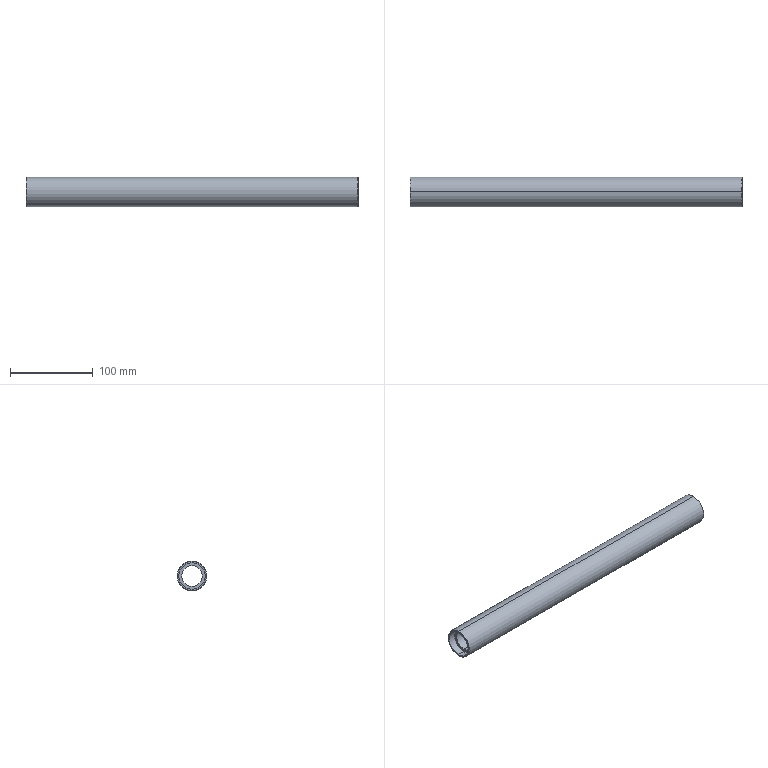Part | STEP file | PN_0018 | 1 solid | 16 faces | box 402 x 36 x 36 mm | volume 206186 mm3 | cylinder 8 | cone 4 | plane 4 | commonest cylinder face diameters 32 x4 25 x2 36 x2
STEP:
#1=CARTESIAN_POINT('',(0.,0.,0.));
#2=DIRECTION('',(0.,0.,1.));
#3=DIRECTION('',(1.,0.,0.));
#4=AXIS2_PLACEMENT_3D('',#1,#2,#3);
#5=CARTESIAN_POINT('',(-201.,0.,17.5));
#6=VERTEX_POINT('',#5);
#7=CARTESIAN_POINT('',(-201.,0.,-17.5));
#8=VERTEX_POINT('',#7);
#9=CARTESIAN_POINT('',(-201.,0.,0.));
#10=DIRECTION('',(-1.,0.,0.));
#11=DIRECTION('',(0.,0.,-1.));
#12=AXIS2_PLACEMENT_3D('',#9,#10,#11);
#13=CIRCLE('',#12,17.5);
#14=CARTESIAN_POINT('',(-201.,0.,0.));
#15=DIRECTION('',(1.,0.,0.));
#16=DIRECTION('',(0.,0.,-1.));
#17=AXIS2_PLACEMENT_3D('',#14,#15,#16);
#18=CONICAL_SURFACE('',#17,17.5,0.7854);
#19=CARTESIAN_POINT('',(6.283,0.));
#20=DIRECTION('',(-1.,0.));
#21=VECTOR('',#20,1.);
#22=LINE('',#19,#21);
#23=(GEOMETRIC_REPRESENTATION_CONTEXT(2)PARAMETRIC_REPRESENTATION_CONTEXT()REPRESENTATION_CONTEXT('',''));
#24=DEFINITIONAL_REPRESENTATION('',(#22),#23);
#25=PCURVE('',#18,#24);
#26=CARTESIAN_POINT('',(-201.,18.,0.));
#27=DIRECTION('',(1.,0.,0.));
#28=DIRECTION('',(0.,0.,-1.));
#29=AXIS2_PLACEMENT_3D('',#26,#27,#28);
#30=PLANE('',#29);
#31=CARTESIAN_POINT('',(17.5,-18.));
#32=CARTESIAN_POINT('',(17.5,-48.311));
#33=CARTESIAN_POINT('',(-8.75,-33.155));
#34=CARTESIAN_POINT('',(-35.,-18.));
#35=CARTESIAN_POINT('',(-8.75,-2.845));
#36=CARTESIAN_POINT('',(17.5,12.311));
#37=CARTESIAN_POINT('',(17.5,-18.));
#38=(BOUNDED_CURVE()B_SPLINE_CURVE(2,(#31,#32,#33,#34,#35,#36,#37),.UNSPECIFIED.,.T.,.F.)B_SPLINE_CURVE_WITH_KNOTS((1,2,2,2,2,1),(-2.094,0.,2.094,4.189,6.283,8.378),.UNSPECIFIED.)CURVE()GEOMETRIC_REPRESENTATION_ITEM()RATIONAL_B_SPLINE_CURVE((1.,0.5,1.,0.5,1.,0.5,1.))REPRESENTATION_ITEM(''));
#39=(GEOMETRIC_REPRESENTATION_CONTEXT(2)PARAMETRIC_REPRESENTATION_CONTEXT()REPRESENTATION_CONTEXT('',''));
#40=DEFINITIONAL_REPRESENTATION('',(#38),#39);
#41=PCURVE('',#30,#40);
#42=SURFACE_CURVE('',#13,(#25,#41),.PCURVE_S1.);
#43=EDGE_CURVE('',#6,#8,#42,.T.);
#44=ORIENTED_EDGE('',*,*,#43,.F.);
#45=CARTESIAN_POINT('',(-200.5,0.,18.));
#46=VERTEX_POINT('',#45);
#47=CARTESIAN_POINT('',(-201.,0.,17.5));
#48=DIRECTION('',(0.7071,0.,0.7071));
#49=VECTOR('',#48,1.);
#50=LINE('',#47,#49);
#51=CARTESIAN_POINT('',(3.142,0.));
#52=DIRECTION('',(0.,1.));
#53=VECTOR('',#52,1.);
#54=LINE('',#51,#53);
#55=(GEOMETRIC_REPRESENTATION_CONTEXT(2)PARAMETRIC_REPRESENTATION_CONTEXT()REPRESENTATION_CONTEXT('',''));
#56=DEFINITIONAL_REPRESENTATION('',(#54),#55);
#57=PCURVE('',#18,#56);
#58=CARTESIAN_POINT('',(-201.,0.,0.));
#59=DIRECTION('',(1.,0.,0.));
#60=DIRECTION('',(0.,0.,-1.));
#61=AXIS2_PLACEMENT_3D('',#58,#59,#60);
#62=CONICAL_SURFACE('',#61,17.5,0.7854);
#63=CARTESIAN_POINT('',(3.142,0.));
#64=DIRECTION('',(0.,1.));
#65=VECTOR('',#64,1.);
#66=LINE('',#63,#65);
#67=(GEOMETRIC_REPRESENTATION_CONTEXT(2)PARAMETRIC_REPRESENTATION_CONTEXT()REPRESENTATION_CONTEXT('',''));
#68=DEFINITIONAL_REPRESENTATION('',(#66),#67);
#69=PCURVE('',#62,#68);
#70=SURFACE_CURVE('',#50,(#57,#69),.PCURVE_S1.);
#71=EDGE_CURVE('',#6,#46,#70,.T.);
#72=ORIENTED_EDGE('',*,*,#71,.T.);
#73=CARTESIAN_POINT('',(-200.5,0.,-18.));
#74=VERTEX_POINT('',#73);
#75=CARTESIAN_POINT('',(-200.5,0.,0.));
#76=DIRECTION('',(1.,0.,0.));
#77=DIRECTION('',(0.,0.,-1.));
#78=AXIS2_PLACEMENT_3D('',#75,#76,#77);
#79=CIRCLE('',#78,18.);
#80=CARTESIAN_POINT('',(0.,0.5));
#81=DIRECTION('',(1.,0.));
#82=VECTOR('',#81,1.);
#83=LINE('',#80,#82);
#84=(GEOMETRIC_REPRESENTATION_CONTEXT(2)PARAMETRIC_REPRESENTATION_CONTEXT()REPRESENTATION_CONTEXT('',''));
#85=DEFINITIONAL_REPRESENTATION('',(#83),#84);
#86=PCURVE('',#18,#85);
#87=CARTESIAN_POINT('',(0.,0.,0.));
#88=DIRECTION('',(-1.,0.,0.));
#89=DIRECTION('',(0.,0.,1.));
#90=AXIS2_PLACEMENT_3D('',#87,#88,#89);
#91=CYLINDRICAL_SURFACE('',#90,18.);
#92=CARTESIAN_POINT('',(3.142,200.5));
#93=DIRECTION('',(-1.,0.));
#94=VECTOR('',#93,1.);
#95=LINE('',#92,#94);
#96=(GEOMETRIC_REPRESENTATION_CONTEXT(2)PARAMETRIC_REPRESENTATION_CONTEXT()REPRESENTATION_CONTEXT('',''));
#97=DEFINITIONAL_REPRESENTATION('',(#95),#96);
#98=PCURVE('',#91,#97);
#99=SURFACE_CURVE('',#79,(#86,#98),.PCURVE_S1.);
#100=EDGE_CURVE('',#74,#46,#99,.T.);
#101=ORIENTED_EDGE('',*,*,#100,.F.);
#102=CARTESIAN_POINT('',(-201.,0.,-17.5));
#103=DIRECTION('',(0.7071,0.,-0.7071));
#104=VECTOR('',#103,1.);
#105=LINE('',#102,#104);
#106=CARTESIAN_POINT('',(0.,0.));
#107=DIRECTION('',(0.,1.));
#108=VECTOR('',#107,1.);
#109=LINE('',#106,#108);
#110=(GEOMETRIC_REPRESENTATION_CONTEXT(2)PARAMETRIC_REPRESENTATION_CONTEXT()REPRESENTATION_CONTEXT('',''));
#111=DEFINITIONAL_REPRESENTATION('',(#109),#110);
#112=PCURVE('',#18,#111);
#113=CARTESIAN_POINT('',(6.283,0.));
#114=DIRECTION('',(0.,1.));
#115=VECTOR('',#114,1.);
#116=LINE('',#113,#115);
#117=(GEOMETRIC_REPRESENTATION_CONTEXT(2)PARAMETRIC_REPRESENTATION_CONTEXT()REPRESENTATION_CONTEXT('',''));
#118=DEFINITIONAL_REPRESENTATION('',(#116),#117);
#119=PCURVE('',#62,#118);
#120=SURFACE_CURVE('',#105,(#112,#119),.PCURVE_S1.);
#121=EDGE_CURVE('',#8,#74,#120,.T.);
#122=ORIENTED_EDGE('',*,*,#121,.F.);
#123=EDGE_LOOP('',(#44,#72,#101,#122));
#124=FACE_BOUND('',#123,.T.);
#125=ADVANCED_FACE('',(#124),#18,.T.);
#126=CARTESIAN_POINT('',(201.,0.,-17.5));
#127=VERTEX_POINT('',#126);
#128=CARTESIAN_POINT('',(201.,0.,17.5));
#129=VERTEX_POINT('',#128);
#130=CARTESIAN_POINT('',(201.,0.,0.));
#131=DIRECTION('',(1.,0.,0.));
#132=DIRECTION('',(0.,0.,1.));
#133=AXIS2_PLACEMENT_3D('',#130,#131,#132);
#134=CIRCLE('',#133,17.5);
#135=CARTESIAN_POINT('',(200.5,0.,0.));
#136=DIRECTION('',(-1.,0.,0.));
#137=DIRECTION('',(0.,0.,1.));
#138=AXIS2_PLACEMENT_3D('',#135,#136,#137);
#139=CONICAL_SURFACE('',#138,18.,0.7854);
#140=CARTESIAN_POINT('',(6.283,-0.5));
#141=DIRECTION('',(-1.,0.));
#142=VECTOR('',#141,1.);
#143=LINE('',#140,#142);
#144=(GEOMETRIC_REPRESENTATION_CONTEXT(2)PARAMETRIC_REPRESENTATION_CONTEXT()REPRESENTATION_CONTEXT('',''));
#145=DEFINITIONAL_REPRESENTATION('',(#143),#144);
#146=PCURVE('',#139,#145);
#147=CARTESIAN_POINT('',(201.,18.,0.));
#148=DIRECTION('',(-1.,0.,0.));
#149=DIRECTION('',(0.,0.,1.));
#150=AXIS2_PLACEMENT_3D('',#147,#148,#149);
#151=PLANE('',#150);
#152=CARTESIAN_POINT('',(17.5,-18.));
#153=CARTESIAN_POINT('',(17.5,-48.311));
#154=CARTESIAN_POINT('',(-8.75,-33.155));
#155=CARTESIAN_POINT('',(-35.,-18.));
#156=CARTESIAN_POINT('',(-8.75,-2.845));
#157=CARTESIAN_POINT('',(17.5,12.311));
#158=CARTESIAN_POINT('',(17.5,-18.));
#159=(BOUNDED_CURVE()B_SPLINE_CURVE(2,(#152,#153,#154,#155,#156,#157,#158),.UNSPECIFIED.,.T.,.F.)B_SPLINE_CURVE_WITH_KNOTS((1,2,2,2,2,1),(-2.094,0.,2.094,4.189,6.283,8.378),.UNSPECIFIED.)CURVE()GEOMETRIC_REPRESENTATION_ITEM()RATIONAL_B_SPLINE_CURVE((1.,0.5,1.,0.5,1.,0.5,1.))REPRESENTATION_ITEM(''));
#160=(GEOMETRIC_REPRESENTATION_CONTEXT(2)PARAMETRIC_REPRESENTATION_CONTEXT()REPRESENTATION_CONTEXT('',''));
#161=DEFINITIONAL_REPRESENTATION('',(#159),#160);
#162=PCURVE('',#151,#161);
#163=SURFACE_CURVE('',#134,(#146,#162),.PCURVE_S1.);
#164=EDGE_CURVE('',#127,#129,#163,.T.);
#165=ORIENTED_EDGE('',*,*,#164,.F.);
#166=CARTESIAN_POINT('',(200.5,0.,-18.));
#167=VERTEX_POINT('',#166);
#168=CARTESIAN_POINT('',(200.5,0.,-18.));
#169=DIRECTION('',(-0.7071,0.,-0.7071));
#170=VECTOR('',#169,1.);
#171=LINE('',#168,#170);
#172=CARTESIAN_POINT('',(3.142,0.));
#173=DIRECTION('',(0.,1.));
#174=VECTOR('',#173,1.);
#175=LINE('',#172,#174);
#176=(GEOMETRIC_REPRESENTATION_CONTEXT(2)PARAMETRIC_REPRESENTATION_CONTEXT()REPRESENTATION_CONTEXT('',''));
#177=DEFINITIONAL_REPRESENTATION('',(#175),#176);
#178=PCURVE('',#139,#177);
#179=CARTESIAN_POINT('',(200.5,0.,0.));
#180=DIRECTION('',(-1.,0.,0.));
#181=DIRECTION('',(0.,0.,1.));
#182=AXIS2_PLACEMENT_3D('',#179,#180,#181);
#183=CONICAL_SURFACE('',#182,18.,0.7854);
#184=CARTESIAN_POINT('',(3.142,0.));
#185=DIRECTION('',(0.,1.));
#186=VECTOR('',#185,1.);
#187=LINE('',#184,#186);
#188=(GEOMETRIC_REPRESENTATION_CONTEXT(2)PARAMETRIC_REPRESENTATION_CONTEXT()REPRESENTATION_CONTEXT('',''));
#189=DEFINITIONAL_REPRESENTATION('',(#187),#188);
#190=PCURVE('',#183,#189);
#191=SURFACE_CURVE('',#171,(#178,#190),.PCURVE_S1.);
#192=EDGE_CURVE('',#127,#167,#191,.T.);
#193=ORIENTED_EDGE('',*,*,#192,.T.);
#194=CARTESIAN_POINT('',(200.5,0.,18.));
#195=VERTEX_POINT('',#194);
#196=CARTESIAN_POINT('',(200.5,0.,0.));
#197=DIRECTION('',(-1.,0.,0.));
#198=DIRECTION('',(0.,0.,1.));
#199=AXIS2_PLACEMENT_3D('',#196,#197,#198);
#200=CIRCLE('',#199,18.);
#201=CARTESIAN_POINT('',(0.,0.));
#202=DIRECTION('',(1.,0.));
#203=VECTOR('',#202,1.);
#204=LINE('',#201,#203);
#205=(GEOMETRIC_REPRESENTATION_CONTEXT(2)PARAMETRIC_REPRESENTATION_CONTEXT()REPRESENTATION_CONTEXT('',''));
#206=DEFINITIONAL_REPRESENTATION('',(#204),#205);
#207=PCURVE('',#139,#206);
#208=CARTESIAN_POINT('',(0.,-200.5));
#209=DIRECTION('',(1.,0.));
#210=VECTOR('',#209,1.);
#211=LINE('',#208,#210);
#212=(GEOMETRIC_REPRESENTATION_CONTEXT(2)PARAMETRIC_REPRESENTATION_CONTEXT()REPRESENTATION_CONTEXT('',''));
#213=DEFINITIONAL_REPRESENTATION('',(#211),#212);
#214=PCURVE('',#91,#213);
#215=SURFACE_CURVE('',#200,(#207,#214),.PCURVE_S1.);
#216=EDGE_CURVE('',#195,#167,#215,.T.);
#217=ORIENTED_EDGE('',*,*,#216,.F.);
#218=CARTESIAN_POINT('',(200.5,0.,18.));
#219=DIRECTION('',(-0.7071,0.,0.7071));
#220=VECTOR('',#219,1.);
#221=LINE('',#218,#220);
#222=CARTESIAN_POINT('',(0.,0.));
#223=DIRECTION('',(0.,1.));
#224=VECTOR('',#223,1.);
#225=LINE('',#222,#224);
#226=(GEOMETRIC_REPRESENTATION_CONTEXT(2)PARAMETRIC_REPRESENTATION_CONTEXT()REPRESENTATION_CONTEXT('',''));
#227=DEFINITIONAL_REPRESENTATION('',(#225),#226);
#228=PCURVE('',#139,#227);
#229=CARTESIAN_POINT('',(6.283,0.));
#230=DIRECTION('',(0.,1.));
#231=VECTOR('',#230,1.);
#232=LINE('',#229,#231);
#233=(GEOMETRIC_REPRESENTATION_CONTEXT(2)PARAMETRIC_REPRESENTATION_CONTEXT()REPRESENTATION_CONTEXT('',''));
#234=DEFINITIONAL_REPRESENTATION('',(#232),#233);
#235=PCURVE('',#183,#234);
#236=SURFACE_CURVE('',#221,(#228,#235),.PCURVE_S1.);
#237=EDGE_CURVE('',#129,#195,#236,.T.);
#238=ORIENTED_EDGE('',*,*,#237,.F.);
#239=EDGE_LOOP('',(#165,#193,#217,#238));
#240=FACE_BOUND('',#239,.T.);
#241=ADVANCED_FACE('',(#240),#139,.T.);
#242=CARTESIAN_POINT('',(192.,0.,12.5));
#243=VERTEX_POINT('',#242);
#244=CARTESIAN_POINT('',(-192.,0.,12.5));
#245=VERTEX_POINT('',#244);
#246=CARTESIAN_POINT('',(0.,0.,12.5));
#247=DIRECTION('',(-1.,0.,0.));
#248=VECTOR('',#247,1.);
#249=LINE('',#246,#248);
#250=CARTESIAN_POINT('',(0.,0.,0.));
#251=DIRECTION('',(-1.,0.,0.));
#252=DIRECTION('',(0.,0.,1.));
#253=AXIS2_PLACEMENT_3D('',#250,#251,#252);
#254=CYLINDRICAL_SURFACE('',#253,12.5);
#255=CARTESIAN_POINT('',(6.283,0.));
#256=DIRECTION('',(0.,1.));
#257=VECTOR('',#256,1.);
#258=LINE('',#255,#257);
#259=(GEOMETRIC_REPRESENTATION_CONTEXT(2)PARAMETRIC_REPRESENTATION_CONTEXT()REPRESENTATION_CONTEXT('',''));
#260=DEFINITIONAL_REPRESENTATION('',(#258),#259);
#261=PCURVE('',#254,#260);
#262=CARTESIAN_POINT('',(0.,0.,0.));
#263=DIRECTION('',(-1.,0.,0.));
#264=DIRECTION('',(0.,0.,1.));
#265=AXIS2_PLACEMENT_3D('',#262,#263,#264);
#266=CYLINDRICAL_SURFACE('',#265,12.5);
#267=CARTESIAN_POINT('',(0.,0.));
#268=DIRECTION('',(0.,1.));
#269=VECTOR('',#268,1.);
#270=LINE('',#267,#269);
#271=(GEOMETRIC_REPRESENTATION_CONTEXT(2)PARAMETRIC_REPRESENTATION_CONTEXT()REPRESENTATION_CONTEXT('',''));
#272=DEFINITIONAL_REPRESENTATION('',(#270),#271);
#273=PCURVE('',#266,#272);
#274=SURFACE_CURVE('',#249,(#261,#273),.PCURVE_S1.);
#275=EDGE_CURVE('',#243,#245,#274,.T.);
#276=ORIENTED_EDGE('',*,*,#275,.T.);
#277=CARTESIAN_POINT('',(-192.,0.,-12.5));
#278=VERTEX_POINT('',#277);
#279=CARTESIAN_POINT('',(-192.,0.,0.));
#280=DIRECTION('',(-1.,0.,0.));
#281=DIRECTION('',(0.,0.,1.));
#282=AXIS2_PLACEMENT_3D('',#279,#280,#281);
#283=CIRCLE('',#282,12.5);
#284=CARTESIAN_POINT('',(0.,192.));
#285=DIRECTION('',(1.,0.));
#286=VECTOR('',#285,1.);
#287=LINE('',#284,#286);
#288=(GEOMETRIC_REPRESENTATION_CONTEXT(2)PARAMETRIC_REPRESENTATION_CONTEXT()REPRESENTATION_CONTEXT('',''));
#289=DEFINITIONAL_REPRESENTATION('',(#287),#288);
#290=PCURVE('',#254,#289);
#291=CARTESIAN_POINT('',(-192.,16.,0.));
#292=DIRECTION('',(1.,0.,0.));
#293=DIRECTION('',(0.,0.,-1.));
#294=AXIS2_PLACEMENT_3D('',#291,#292,#293);
#295=PLANE('',#294);
#296=CARTESIAN_POINT('',(-12.5,-16.));
#297=CARTESIAN_POINT('',(-12.5,5.651));
#298=CARTESIAN_POINT('',(6.25,-5.175));
#299=CARTESIAN_POINT('',(25.,-16.));
#300=CARTESIAN_POINT('',(6.25,-26.825));
#301=CARTESIAN_POINT('',(-12.5,-37.651));
#302=CARTESIAN_POINT('',(-12.5,-16.));
#303=(BOUNDED_CURVE()B_SPLINE_CURVE(2,(#296,#297,#298,#299,#300,#301,#302),.UNSPECIFIED.,.T.,.F.)B_SPLINE_CURVE_WITH_KNOTS((1,2,2,2,2,1),(-2.094,0.,2.094,4.189,6.283,8.378),.UNSPECIFIED.)CURVE()GEOMETRIC_REPRESENTATION_ITEM()RATIONAL_B_SPLINE_CURVE((1.,0.5,1.,0.5,1.,0.5,1.))REPRESENTATION_ITEM(''));
#304=(GEOMETRIC_REPRESENTATION_CONTEXT(2)PARAMETRIC_REPRESENTATION_CONTEXT()REPRESENTATION_CONTEXT('',''));
#305=DEFINITIONAL_REPRESENTATION('',(#303),#304);
#306=PCURVE('',#295,#305);
#307=SURFACE_CURVE('',#283,(#290,#306),.PCURVE_S1.);
#308=EDGE_CURVE('',#278,#245,#307,.T.);
#309=ORIENTED_EDGE('',*,*,#308,.F.);
#310=CARTESIAN_POINT('',(192.,0.,-12.5));
#311=VERTEX_POINT('',#310);
#312=CARTESIAN_POINT('',(0.,0.,-12.5));
#313=DIRECTION('',(-1.,0.,0.));
#314=VECTOR('',#313,1.);
#315=LINE('',#312,#314);
#316=CARTESIAN_POINT('',(3.142,0.));
#317=DIRECTION('',(0.,1.));
#318=VECTOR('',#317,1.);
#319=LINE('',#316,#318);
#320=(GEOMETRIC_REPRESENTATION_CONTEXT(2)PARAMETRIC_REPRESENTATION_CONTEXT()REPRESENTATION_CONTEXT('',''));
#321=DEFINITIONAL_REPRESENTATION('',(#319),#320);
#322=PCURVE('',#254,#321);
#323=CARTESIAN_POINT('',(3.142,0.));
#324=DIRECTION('',(0.,1.));
#325=VECTOR('',#324,1.);
#326=LINE('',#323,#325);
#327=(GEOMETRIC_REPRESENTATION_CONTEXT(2)PARAMETRIC_REPRESENTATION_CONTEXT()REPRESENTATION_CONTEXT('',''));
#328=DEFINITIONAL_REPRESENTATION('',(#326),#327);
#329=PCURVE('',#266,#328);
#330=SURFACE_CURVE('',#315,(#322,#329),.PCURVE_S1.);
#331=EDGE_CURVE('',#311,#278,#330,.T.);
#332=ORIENTED_EDGE('',*,*,#331,.F.);
#333=CARTESIAN_POINT('',(192.,0.,0.));
#334=DIRECTION('',(-1.,0.,0.));
#335=DIRECTION('',(0.,0.,1.));
#336=AXIS2_PLACEMENT_3D('',#333,#334,#335);
#337=CIRCLE('',#336,12.5);
#338=CARTESIAN_POINT('',(0.,-192.));
#339=DIRECTION('',(1.,0.));
#340=VECTOR('',#339,1.);
#341=LINE('',#338,#340);
#342=(GEOMETRIC_REPRESENTATION_CONTEXT(2)PARAMETRIC_REPRESENTATION_CONTEXT()REPRESENTATION_CONTEXT('',''));
#343=DEFINITIONAL_REPRESENTATION('',(#341),#342);
#344=PCURVE('',#254,#343);
#345=CARTESIAN_POINT('',(192.,16.,0.));
#346=DIRECTION('',(-1.,0.,0.));
#347=DIRECTION('',(0.,0.,1.));
#348=AXIS2_PLACEMENT_3D('',#345,#346,#347);
#349=PLANE('',#348);
#350=CARTESIAN_POINT('',(0.,-16.));
#351=DIRECTION('',(1.,0.));
#352=AXIS2_PLACEMENT_2D('',#350,#351);
#353=CIRCLE('',#352,12.5);
#354=(GEOMETRIC_REPRESENTATION_CONTEXT(2)PARAMETRIC_REPRESENTATION_CONTEXT()REPRESENTATION_CONTEXT('',''));
#355=DEFINITIONAL_REPRESENTATION('',(#353),#354);
#356=PCURVE('',#349,#355);
#357=SURFACE_CURVE('',#337,(#344,#356),.PCURVE_S1.);
#358=EDGE_CURVE('',#311,#243,#357,.T.);
#359=ORIENTED_EDGE('',*,*,#358,.T.);
#360=EDGE_LOOP('',(#276,#309,#332,#359));
#361=FACE_BOUND('',#360,.F.);
#362=ADVANCED_FACE('',(#361),#254,.F.);
#363=CARTESIAN_POINT('',(201.,0.,16.));
#364=VERTEX_POINT('',#363);
#365=CARTESIAN_POINT('',(192.,0.,16.));
#366=VERTEX_POINT('',#365);
#367=CARTESIAN_POINT('',(0.,0.,16.));
#368=DIRECTION('',(-1.,0.,0.));
#369=VECTOR('',#368,1.);
#370=LINE('',#367,#369);
#371=CARTESIAN_POINT('',(0.,0.,0.));
#372=DIRECTION('',(-1.,0.,0.));
#373=DIRECTION('',(0.,0.,1.));
#374=AXIS2_PLACEMENT_3D('',#371,#372,#373);
#375=CYLINDRICAL_SURFACE('',#374,16.);
#376=CARTESIAN_POINT('',(6.283,0.));
#377=DIRECTION('',(0.,1.));
#378=VECTOR('',#377,1.);
#379=LINE('',#376,#378);
#380=(GEOMETRIC_REPRESENTATION_CONTEXT(2)PARAMETRIC_REPRESENTATION_CONTEXT()REPRESENTATION_CONTEXT('',''));
#381=DEFINITIONAL_REPRESENTATION('',(#379),#380);
#382=PCURVE('',#375,#381);
#383=CARTESIAN_POINT('',(0.,0.,0.));
#384=DIRECTION('',(-1.,0.,0.));
#385=DIRECTION('',(0.,0.,1.));
#386=AXIS2_PLACEMENT_3D('',#383,#384,#385);
#387=CYLINDRICAL_SURFACE('',#386,16.);
#388=CARTESIAN_POINT('',(0.,0.));
#389=DIRECTION('',(0.,1.));
#390=VECTOR('',#389,1.);
#391=LINE('',#388,#390);
#392=(GEOMETRIC_REPRESENTATION_CONTEXT(2)PARAMETRIC_REPRESENTATION_CONTEXT()REPRESENTATION_CONTEXT('',''));
#393=DEFINITIONAL_REPRESENTATION('',(#391),#392);
#394=PCURVE('',#387,#393);
#395=SURFACE_CURVE('',#370,(#382,#394),.PCURVE_S1.);
#396=EDGE_CURVE('',#364,#366,#395,.T.);
#397=ORIENTED_EDGE('',*,*,#396,.T.);
#398=CARTESIAN_POINT('',(192.,0.,-16.));
#399=VERTEX_POINT('',#398);
#400=CARTESIAN_POINT('',(192.,0.,0.));
#401=DIRECTION('',(-1.,0.,0.));
#402=DIRECTION('',(0.,0.,1.));
#403=AXIS2_PLACEMENT_3D('',#400,#401,#402);
#404=CIRCLE('',#403,16.);
#405=CARTESIAN_POINT('',(0.,-192.));
#406=DIRECTION('',(1.,0.));
#407=VECTOR('',#406,1.);
#408=LINE('',#405,#407);
#409=(GEOMETRIC_REPRESENTATION_CONTEXT(2)PARAMETRIC_REPRESENTATION_CONTEXT()REPRESENTATION_CONTEXT('',''));
#410=DEFINITIONAL_REPRESENTATION('',(#408),#409);
#411=PCURVE('',#375,#410);
#412=CARTESIAN_POINT('',(0.,-16.));
#413=DIRECTION('',(1.,0.));
#414=AXIS2_PLACEMENT_2D('',#412,#413);
#415=CIRCLE('',#414,16.);
#416=(GEOMETRIC_REPRESENTATION_CONTEXT(2)PARAMETRIC_REPRESENTATION_CONTEXT()REPRESENTATION_CONTEXT('',''));
#417=DEFINITIONAL_REPRESENTATION('',(#415),#416);
#418=PCURVE('',#349,#417);
#419=SURFACE_CURVE('',#404,(#411,#418),.PCURVE_S1.);
#420=EDGE_CURVE('',#399,#366,#419,.T.);
#421=ORIENTED_EDGE('',*,*,#420,.F.);
#422=CARTESIAN_POINT('',(201.,0.,-16.));
#423=VERTEX_POINT('',#422);
#424=CARTESIAN_POINT('',(0.,0.,-16.));
#425=DIRECTION('',(-1.,0.,0.));
#426=VECTOR('',#425,1.);
#427=LINE('',#424,#426);
#428=CARTESIAN_POINT('',(3.142,0.));
#429=DIRECTION('',(0.,1.));
#430=VECTOR('',#429,1.);
#431=LINE('',#428,#430);
#432=(GEOMETRIC_REPRESENTATION_CONTEXT(2)PARAMETRIC_REPRESENTATION_CONTEXT()REPRESENTATION_CONTEXT('',''));
#433=DEFINITIONAL_REPRESENTATION('',(#431),#432);
#434=PCURVE('',#375,#433);
#435=CARTESIAN_POINT('',(3.142,0.));
#436=DIRECTION('',(0.,1.));
#437=VECTOR('',#436,1.);
#438=LINE('',#435,#437);
#439=(GEOMETRIC_REPRESENTATION_CONTEXT(2)PARAMETRIC_REPRESENTATION_CONTEXT()REPRESENTATION_CONTEXT('',''));
#440=DEFINITIONAL_REPRESENTATION('',(#438),#439);
#441=PCURVE('',#387,#440);
#442=SURFACE_CURVE('',#427,(#434,#441),.PCURVE_S1.);
#443=EDGE_CURVE('',#423,#399,#442,.T.);
#444=ORIENTED_EDGE('',*,*,#443,.F.);
#445=CARTESIAN_POINT('',(201.,0.,0.));
#446=DIRECTION('',(-1.,0.,0.));
#447=DIRECTION('',(0.,0.,1.));
#448=AXIS2_PLACEMENT_3D('',#445,#446,#447);
#449=CIRCLE('',#448,16.);
#450=CARTESIAN_POINT('',(0.,-201.));
#451=DIRECTION('',(1.,0.));
#452=VECTOR('',#451,1.);
#453=LINE('',#450,#452);
#454=(GEOMETRIC_REPRESENTATION_CONTEXT(2)PARAMETRIC_REPRESENTATION_CONTEXT()REPRESENTATION_CONTEXT('',''));
#455=DEFINITIONAL_REPRESENTATION('',(#453),#454);
#456=PCURVE('',#375,#455);
#457=CARTESIAN_POINT('',(0.,-18.));
#458=DIRECTION('',(1.,0.));
#459=AXIS2_PLACEMENT_2D('',#457,#458);
#460=CIRCLE('',#459,16.);
#461=(GEOMETRIC_REPRESENTATION_CONTEXT(2)PARAMETRIC_REPRESENTATION_CONTEXT()REPRESENTATION_CONTEXT('',''));
#462=DEFINITIONAL_REPRESENTATION('',(#460),#461);
#463=PCURVE('',#151,#462);
#464=SURFACE_CURVE('',#449,(#456,#463),.PCURVE_S1.);
#465=EDGE_CURVE('',#423,#364,#464,.T.);
#466=ORIENTED_EDGE('',*,*,#465,.T.);
#467=EDGE_LOOP('',(#397,#421,#444,#466));
#468=FACE_BOUND('',#467,.F.);
#469=ADVANCED_FACE('',(#468),#375,.F.);
#470=ORIENTED_EDGE('',*,*,#216,.T.);
#471=CARTESIAN_POINT('',(0.,0.,-18.));
#472=DIRECTION('',(-1.,0.,0.));
#473=VECTOR('',#472,1.);
#474=LINE('',#471,#473);
#475=CARTESIAN_POINT('',(3.142,0.));
#476=DIRECTION('',(0.,1.));
#477=VECTOR('',#476,1.);
#478=LINE('',#475,#477);
#479=(GEOMETRIC_REPRESENTATION_CONTEXT(2)PARAMETRIC_REPRESENTATION_CONTEXT()REPRESENTATION_CONTEXT('',''));
#480=DEFINITIONAL_REPRESENTATION('',(#478),#479);
#481=PCURVE('',#91,#480);
#482=CARTESIAN_POINT('',(0.,0.,0.));
#483=DIRECTION('',(-1.,0.,0.));
#484=DIRECTION('',(0.,0.,1.));
#485=AXIS2_PLACEMENT_3D('',#482,#483,#484);
#486=CYLINDRICAL_SURFACE('',#485,18.);
#487=CARTESIAN_POINT('',(3.142,0.));
#488=DIRECTION('',(0.,1.));
#489=VECTOR('',#488,1.);
#490=LINE('',#487,#489);
#491=(GEOMETRIC_REPRESENTATION_CONTEXT(2)PARAMETRIC_REPRESENTATION_CONTEXT()REPRESENTATION_CONTEXT('',''));
#492=DEFINITIONAL_REPRESENTATION('',(#490),#491);
#493=PCURVE('',#486,#492);
#494=SURFACE_CURVE('',#474,(#481,#493),.PCURVE_S1.);
#495=EDGE_CURVE('',#167,#74,#494,.T.);
#496=ORIENTED_EDGE('',*,*,#495,.T.);
#497=ORIENTED_EDGE('',*,*,#100,.T.);
#498=CARTESIAN_POINT('',(0.,0.,18.));
#499=DIRECTION('',(-1.,0.,0.));
#500=VECTOR('',#499,1.);
#501=LINE('',#498,#500);
#502=CARTESIAN_POINT('',(0.,0.));
#503=DIRECTION('',(0.,1.));
#504=VECTOR('',#503,1.);
#505=LINE('',#502,#504);
#506=(GEOMETRIC_REPRESENTATION_CONTEXT(2)PARAMETRIC_REPRESENTATION_CONTEXT()REPRESENTATION_CONTEXT('',''));
#507=DEFINITIONAL_REPRESENTATION('',(#505),#506);
#508=PCURVE('',#91,#507);
#509=CARTESIAN_POINT('',(6.283,0.));
#510=DIRECTION('',(0.,1.));
#511=VECTOR('',#510,1.);
#512=LINE('',#509,#511);
#513=(GEOMETRIC_REPRESENTATION_CONTEXT(2)PARAMETRIC_REPRESENTATION_CONTEXT()REPRESENTATION_CONTEXT('',''));
#514=DEFINITIONAL_REPRESENTATION('',(#512),#513);
#515=PCURVE('',#486,#514);
#516=SURFACE_CURVE('',#501,(#508,#515),.PCURVE_S1.);
#517=EDGE_CURVE('',#195,#46,#516,.T.);
#518=ORIENTED_EDGE('',*,*,#517,.F.);
#519=EDGE_LOOP('',(#470,#496,#497,#518));
#520=FACE_BOUND('',#519,.T.);
#521=ADVANCED_FACE('',(#520),#91,.T.);
#522=CARTESIAN_POINT('',(-192.,0.,16.));
#523=VERTEX_POINT('',#522);
#524=CARTESIAN_POINT('',(-201.,0.,16.));
#525=VERTEX_POINT('',#524);
#526=CARTESIAN_POINT('',(0.,0.,16.));
#527=DIRECTION('',(-1.,0.,0.));
#528=VECTOR('',#527,1.);
#529=LINE('',#526,#528);
#530=CARTESIAN_POINT('',(0.,0.,0.));
#531=DIRECTION('',(-1.,0.,0.));
#532=DIRECTION('',(0.,0.,1.));
#533=AXIS2_PLACEMENT_3D('',#530,#531,#532);
#534=CYLINDRICAL_SURFACE('',#533,16.);
#535=CARTESIAN_POINT('',(6.283,0.));
#536=DIRECTION('',(0.,1.));
#537=VECTOR('',#536,1.);
#538=LINE('',#535,#537);
#539=(GEOMETRIC_REPRESENTATION_CONTEXT(2)PARAMETRIC_REPRESENTATION_CONTEXT()REPRESENTATION_CONTEXT('',''));
#540=DEFINITIONAL_REPRESENTATION('',(#538),#539);
#541=PCURVE('',#534,#540);
#542=CARTESIAN_POINT('',(0.,0.,0.));
#543=DIRECTION('',(-1.,0.,0.));
#544=DIRECTION('',(0.,0.,1.));
#545=AXIS2_PLACEMENT_3D('',#542,#543,#544);
#546=CYLINDRICAL_SURFACE('',#545,16.);
#547=CARTESIAN_POINT('',(0.,0.));
#548=DIRECTION('',(0.,1.));
#549=VECTOR('',#548,1.);
#550=LINE('',#547,#549);
#551=(GEOMETRIC_REPRESENTATION_CONTEXT(2)PARAMETRIC_REPRESENTATION_CONTEXT()REPRESENTATION_CONTEXT('',''));
#552=DEFINITIONAL_REPRESENTATION('',(#550),#551);
#553=PCURVE('',#546,#552);
#554=SURFACE_CURVE('',#529,(#541,#553),.PCURVE_S1.);
#555=EDGE_CURVE('',#523,#525,#554,.T.);
#556=ORIENTED_EDGE('',*,*,#555,.T.);
#557=CARTESIAN_POINT('',(-201.,0.,-16.));
#558=VERTEX_POINT('',#557);
#559=CARTESIAN_POINT('',(-201.,0.,0.));
#560=DIRECTION('',(-1.,0.,0.));
#561=DIRECTION('',(0.,0.,1.));
#562=AXIS2_PLACEMENT_3D('',#559,#560,#561);
#563=CIRCLE('',#562,16.);
#564=CARTESIAN_POINT('',(0.,201.));
#565=DIRECTION('',(1.,0.));
#566=VECTOR('',#565,1.);
#567=LINE('',#564,#566);
#568=(GEOMETRIC_REPRESENTATION_CONTEXT(2)PARAMETRIC_REPRESENTATION_CONTEXT()REPRESENTATION_CONTEXT('',''));
#569=DEFINITIONAL_REPRESENTATION('',(#567),#568);
#570=PCURVE('',#534,#569);
#571=CARTESIAN_POINT('',(-16.,-18.));
#572=CARTESIAN_POINT('',(-16.,9.713));
#573=CARTESIAN_POINT('',(8.,-4.144));
#574=CARTESIAN_POINT('',(32.,-18.));
#575=CARTESIAN_POINT('',(8.,-31.856));
#576=CARTESIAN_POINT('',(-16.,-45.713));
#577=CARTESIAN_POINT('',(-16.,-18.));
#578=(BOUNDED_CURVE()B_SPLINE_CURVE(2,(#571,#572,#573,#574,#575,#576,#577),.UNSPECIFIED.,.T.,.F.)B_SPLINE_CURVE_WITH_KNOTS((1,2,2,2,2,1),(-2.094,0.,2.094,4.189,6.283,8.378),.UNSPECIFIED.)CURVE()GEOMETRIC_REPRESENTATION_ITEM()RATIONAL_B_SPLINE_CURVE((1.,0.5,1.,0.5,1.,0.5,1.))REPRESENTATION_ITEM(''));
#579=(GEOMETRIC_REPRESENTATION_CONTEXT(2)PARAMETRIC_REPRESENTATION_CONTEXT()REPRESENTATION_CONTEXT('',''));
#580=DEFINITIONAL_REPRESENTATION('',(#578),#579);
#581=PCURVE('',#30,#580);
#582=SURFACE_CURVE('',#563,(#570,#581),.PCURVE_S1.);
#583=EDGE_CURVE('',#558,#525,#582,.T.);
#584=ORIENTED_EDGE('',*,*,#583,.F.);
#585=CARTESIAN_POINT('',(-192.,0.,-16.));
#586=VERTEX_POINT('',#585);
#587=CARTESIAN_POINT('',(0.,0.,-16.));
#588=DIRECTION('',(-1.,0.,0.));
#589=VECTOR('',#588,1.);
#590=LINE('',#587,#589);
#591=CARTESIAN_POINT('',(3.142,0.));
#592=DIRECTION('',(0.,1.));
#593=VECTOR('',#592,1.);
#594=LINE('',#591,#593);
#595=(GEOMETRIC_REPRESENTATION_CONTEXT(2)PARAMETRIC_REPRESENTATION_CONTEXT()REPRESENTATION_CONTEXT('',''));
#596=DEFINITIONAL_REPRESENTATION('',(#594),#595);
#597=PCURVE('',#534,#596);
#598=CARTESIAN_POINT('',(3.142,0.));
#599=DIRECTION('',(0.,1.));
#600=VECTOR('',#599,1.);
#601=LINE('',#598,#600);
#602=(GEOMETRIC_REPRESENTATION_CONTEXT(2)PARAMETRIC_REPRESENTATION_CONTEXT()REPRESENTATION_CONTEXT('',''));
#603=DEFINITIONAL_REPRESENTATION('',(#601),#602);
#604=PCURVE('',#546,#603);
#605=SURFACE_CURVE('',#590,(#597,#604),.PCURVE_S1.);
#606=EDGE_CURVE('',#586,#558,#605,.T.);
#607=ORIENTED_EDGE('',*,*,#606,.F.);
#608=CARTESIAN_POINT('',(-192.,0.,0.));
#609=DIRECTION('',(-1.,0.,0.));
#610=DIRECTION('',(0.,0.,1.));
#611=AXIS2_PLACEMENT_3D('',#608,#609,#610);
#612=CIRCLE('',#611,16.);
#613=CARTESIAN_POINT('',(0.,192.));
#614=DIRECTION('',(1.,0.));
#615=VECTOR('',#614,1.);
#616=LINE('',#613,#615);
#617=(GEOMETRIC_REPRESENTATION_CONTEXT(2)PARAMETRIC_REPRESENTATION_CONTEXT()REPRESENTATION_CONTEXT('',''));
#618=DEFINITIONAL_REPRESENTATION('',(#616),#617);
#619=PCURVE('',#534,#618);
#620=CARTESIAN_POINT('',(-16.,-16.));
#621=CARTESIAN_POINT('',(-16.,11.713));
#622=CARTESIAN_POINT('',(8.,-2.144));
#623=CARTESIAN_POINT('',(32.,-16.));
#624=CARTESIAN_POINT('',(8.,-29.856));
#625=CARTESIAN_POINT('',(-16.,-43.713));
#626=CARTESIAN_POINT('',(-16.,-16.));
#627=(BOUNDED_CURVE()B_SPLINE_CURVE(2,(#620,#621,#622,#623,#624,#625,#626),.UNSPECIFIED.,.T.,.F.)B_SPLINE_CURVE_WITH_KNOTS((1,2,2,2,2,1),(-2.094,0.,2.094,4.189,6.283,8.378),.UNSPECIFIED.)CURVE()GEOMETRIC_REPRESENTATION_ITEM()RATIONAL_B_SPLINE_CURVE((1.,0.5,1.,0.5,1.,0.5,1.))REPRESENTATION_ITEM(''));
#628=(GEOMETRIC_REPRESENTATION_CONTEXT(2)PARAMETRIC_REPRESENTATION_CONTEXT()REPRESENTATION_CONTEXT('',''));
#629=DEFINITIONAL_REPRESENTATION('',(#627),#628);
#630=PCURVE('',#295,#629);
#631=SURFACE_CURVE('',#612,(#619,#630),.PCURVE_S1.);
#632=EDGE_CURVE('',#586,#523,#631,.T.);
#633=ORIENTED_EDGE('',*,*,#632,.T.);
#634=EDGE_LOOP('',(#556,#584,#607,#633));
#635=FACE_BOUND('',#634,.F.);
#636=ADVANCED_FACE('',(#635),#534,.F.);
#637=CARTESIAN_POINT('',(-192.,0.,0.));
#638=DIRECTION('',(-1.,0.,0.));
#639=DIRECTION('',(0.,0.,1.));
#640=AXIS2_PLACEMENT_3D('',#637,#638,#639);
#641=CIRCLE('',#640,12.5);
#642=CARTESIAN_POINT('',(-12.5,-16.));
#643=CARTESIAN_POINT('',(-12.5,5.651));
#644=CARTESIAN_POINT('',(6.25,-5.175));
#645=CARTESIAN_POINT('',(25.,-16.));
#646=CARTESIAN_POINT('',(6.25,-26.825));
#647=CARTESIAN_POINT('',(-12.5,-37.651));
#648=CARTESIAN_POINT('',(-12.5,-16.));
#649=(BOUNDED_CURVE()B_SPLINE_CURVE(2,(#642,#643,#644,#645,#646,#647,#648),.UNSPECIFIED.,.T.,.F.)B_SPLINE_CURVE_WITH_KNOTS((1,2,2,2,2,1),(-2.094,0.,2.094,4.189,6.283,8.378),.UNSPECIFIED.)CURVE()GEOMETRIC_REPRESENTATION_ITEM()RATIONAL_B_SPLINE_CURVE((1.,0.5,1.,0.5,1.,0.5,1.))REPRESENTATION_ITEM(''));
#650=(GEOMETRIC_REPRESENTATION_CONTEXT(2)PARAMETRIC_REPRESENTATION_CONTEXT()REPRESENTATION_CONTEXT('',''));
#651=DEFINITIONAL_REPRESENTATION('',(#649),#650);
#652=PCURVE('',#295,#651);
#653=CARTESIAN_POINT('',(0.,192.));
#654=DIRECTION('',(1.,0.));
#655=VECTOR('',#654,1.);
#656=LINE('',#653,#655);
#657=(GEOMETRIC_REPRESENTATION_CONTEXT(2)PARAMETRIC_REPRESENTATION_CONTEXT()REPRESENTATION_CONTEXT('',''));
#658=DEFINITIONAL_REPRESENTATION('',(#656),#657);
#659=PCURVE('',#266,#658);
#660=SURFACE_CURVE('',#641,(#652,#659),.PCURVE_S1.);
#661=EDGE_CURVE('',#245,#278,#660,.T.);
#662=ORIENTED_EDGE('',*,*,#661,.F.);
#663=ORIENTED_EDGE('',*,*,#308,.F.);
#664=EDGE_LOOP('',(#662,#663));
#665=FACE_BOUND('',#664,.T.);
#666=CARTESIAN_POINT('',(-192.,0.,0.));
#667=DIRECTION('',(-1.,0.,0.));
#668=DIRECTION('',(0.,0.,1.));
#669=AXIS2_PLACEMENT_3D('',#666,#667,#668);
#670=CIRCLE('',#669,16.);
#671=CARTESIAN_POINT('',(-16.,-16.));
#672=CARTESIAN_POINT('',(-16.,11.713));
#673=CARTESIAN_POINT('',(8.,-2.144));
#674=CARTESIAN_POINT('',(32.,-16.));
#675=CARTESIAN_POINT('',(8.,-29.856));
#676=CARTESIAN_POINT('',(-16.,-43.713));
#677=CARTESIAN_POINT('',(-16.,-16.));
#678=(BOUNDED_CURVE()B_SPLINE_CURVE(2,(#671,#672,#673,#674,#675,#676,#677),.UNSPECIFIED.,.T.,.F.)B_SPLINE_CURVE_WITH_KNOTS((1,2,2,2,2,1),(-2.094,0.,2.094,4.189,6.283,8.378),.UNSPECIFIED.)CURVE()GEOMETRIC_REPRESENTATION_ITEM()RATIONAL_B_SPLINE_CURVE((1.,0.5,1.,0.5,1.,0.5,1.))REPRESENTATION_ITEM(''));
#679=(GEOMETRIC_REPRESENTATION_CONTEXT(2)PARAMETRIC_REPRESENTATION_CONTEXT()REPRESENTATION_CONTEXT('',''));
#680=DEFINITIONAL_REPRESENTATION('',(#678),#679);
#681=PCURVE('',#295,#680);
#682=CARTESIAN_POINT('',(0.,192.));
#683=DIRECTION('',(1.,0.));
#684=VECTOR('',#683,1.);
#685=LINE('',#682,#684);
#686=(GEOMETRIC_REPRESENTATION_CONTEXT(2)PARAMETRIC_REPRESENTATION_CONTEXT()REPRESENTATION_CONTEXT('',''));
#687=DEFINITIONAL_REPRESENTATION('',(#685),#686);
#688=PCURVE('',#546,#687);
#689=SURFACE_CURVE('',#670,(#681,#688),.PCURVE_S1.);
#690=EDGE_CURVE('',#523,#586,#689,.T.);
#691=ORIENTED_EDGE('',*,*,#690,.T.);
#692=ORIENTED_EDGE('',*,*,#632,.T.);
#693=EDGE_LOOP('',(#691,#692));
#694=FACE_BOUND('',#693,.T.);
#695=ADVANCED_FACE('',(#665,#694),#295,.F.);
#696=CARTESIAN_POINT('',(-201.,0.,0.));
#697=DIRECTION('',(-1.,0.,0.));
#698=DIRECTION('',(0.,0.,1.));
#699=AXIS2_PLACEMENT_3D('',#696,#697,#698);
#700=CIRCLE('',#699,16.);
#701=CARTESIAN_POINT('',(0.,201.));
#702=DIRECTION('',(1.,0.));
#703=VECTOR('',#702,1.);
#704=LINE('',#701,#703);
#705=(GEOMETRIC_REPRESENTATION_CONTEXT(2)PARAMETRIC_REPRESENTATION_CONTEXT()REPRESENTATION_CONTEXT('',''));
#706=DEFINITIONAL_REPRESENTATION('',(#704),#705);
#707=PCURVE('',#546,#706);
#708=CARTESIAN_POINT('',(-16.,-18.));
#709=CARTESIAN_POINT('',(-16.,9.713));
#710=CARTESIAN_POINT('',(8.,-4.144));
#711=CARTESIAN_POINT('',(32.,-18.));
#712=CARTESIAN_POINT('',(8.,-31.856));
#713=CARTESIAN_POINT('',(-16.,-45.713));
#714=CARTESIAN_POINT('',(-16.,-18.));
#715=(BOUNDED_CURVE()B_SPLINE_CURVE(2,(#708,#709,#710,#711,#712,#713,#714),.UNSPECIFIED.,.T.,.F.)B_SPLINE_CURVE_WITH_KNOTS((1,2,2,2,2,1),(-2.094,0.,2.094,4.189,6.283,8.378),.UNSPECIFIED.)CURVE()GEOMETRIC_REPRESENTATION_ITEM()RATIONAL_B_SPLINE_CURVE((1.,0.5,1.,0.5,1.,0.5,1.))REPRESENTATION_ITEM(''));
#716=(GEOMETRIC_REPRESENTATION_CONTEXT(2)PARAMETRIC_REPRESENTATION_CONTEXT()REPRESENTATION_CONTEXT('',''));
#717=DEFINITIONAL_REPRESENTATION('',(#715),#716);
#718=PCURVE('',#30,#717);
#719=SURFACE_CURVE('',#700,(#707,#718),.PCURVE_S1.);
#720=EDGE_CURVE('',#525,#558,#719,.T.);
#721=ORIENTED_EDGE('',*,*,#720,.F.);
#722=ORIENTED_EDGE('',*,*,#555,.F.);
#723=ORIENTED_EDGE('',*,*,#690,.T.);
#724=ORIENTED_EDGE('',*,*,#606,.T.);
#725=EDGE_LOOP('',(#721,#722,#723,#724));
#726=FACE_BOUND('',#725,.F.);
#727=ADVANCED_FACE('',(#726),#546,.F.);
#728=CARTESIAN_POINT('',(-201.,0.,0.));
#729=DIRECTION('',(-1.,0.,0.));
#730=DIRECTION('',(0.,0.,-1.));
#731=AXIS2_PLACEMENT_3D('',#728,#729,#730);
#732=CIRCLE('',#731,17.5);
#733=CARTESIAN_POINT('',(17.5,-18.));
#734=CARTESIAN_POINT('',(17.5,-48.311));
#735=CARTESIAN_POINT('',(-8.75,-33.155));
#736=CARTESIAN_POINT('',(-35.,-18.));
#737=CARTESIAN_POINT('',(-8.75,-2.845));
#738=CARTESIAN_POINT('',(17.5,12.311));
#739=CARTESIAN_POINT('',(17.5,-18.));
#740=(BOUNDED_CURVE()B_SPLINE_CURVE(2,(#733,#734,#735,#736,#737,#738,#739),.UNSPECIFIED.,.T.,.F.)B_SPLINE_CURVE_WITH_KNOTS((1,2,2,2,2,1),(-2.094,0.,2.094,4.189,6.283,8.378),.UNSPECIFIED.)CURVE()GEOMETRIC_REPRESENTATION_ITEM()RATIONAL_B_SPLINE_CURVE((1.,0.5,1.,0.5,1.,0.5,1.))REPRESENTATION_ITEM(''));
#741=(GEOMETRIC_REPRESENTATION_CONTEXT(2)PARAMETRIC_REPRESENTATION_CONTEXT()REPRESENTATION_CONTEXT('',''));
#742=DEFINITIONAL_REPRESENTATION('',(#740),#741);
#743=PCURVE('',#30,#742);
#744=CARTESIAN_POINT('',(6.283,0.));
#745=DIRECTION('',(-1.,0.));
#746=VECTOR('',#745,1.);
#747=LINE('',#744,#746);
#748=(GEOMETRIC_REPRESENTATION_CONTEXT(2)PARAMETRIC_REPRESENTATION_CONTEXT()REPRESENTATION_CONTEXT('',''));
#749=DEFINITIONAL_REPRESENTATION('',(#747),#748);
#750=PCURVE('',#62,#749);
#751=SURFACE_CURVE('',#732,(#743,#750),.PCURVE_S1.);
#752=EDGE_CURVE('',#8,#6,#751,.T.);
#753=ORIENTED_EDGE('',*,*,#752,.T.);
#754=ORIENTED_EDGE('',*,*,#43,.T.);
#755=EDGE_LOOP('',(#753,#754));
#756=FACE_BOUND('',#755,.T.);
#757=ORIENTED_EDGE('',*,*,#720,.F.);
#758=ORIENTED_EDGE('',*,*,#583,.F.);
#759=EDGE_LOOP('',(#757,#758));
#760=FACE_BOUND('',#759,.T.);
#761=ADVANCED_FACE('',(#756,#760),#30,.F.);
#762=ORIENTED_EDGE('',*,*,#495,.F.);
#763=CARTESIAN_POINT('',(200.5,0.,0.));
#764=DIRECTION('',(-1.,0.,0.));
#765=DIRECTION('',(0.,0.,1.));
#766=AXIS2_PLACEMENT_3D('',#763,#764,#765);
#767=CIRCLE('',#766,18.);
#768=CARTESIAN_POINT('',(0.,-200.5));
#769=DIRECTION('',(1.,0.));
#770=VECTOR('',#769,1.);
#771=LINE('',#768,#770);
#772=(GEOMETRIC_REPRESENTATION_CONTEXT(2)PARAMETRIC_REPRESENTATION_CONTEXT()REPRESENTATION_CONTEXT('',''));
#773=DEFINITIONAL_REPRESENTATION('',(#771),#772);
#774=PCURVE('',#486,#773);
#775=CARTESIAN_POINT('',(0.,0.));
#776=DIRECTION('',(1.,0.));
#777=VECTOR('',#776,1.);
#778=LINE('',#775,#777);
#779=(GEOMETRIC_REPRESENTATION_CONTEXT(2)PARAMETRIC_REPRESENTATION_CONTEXT()REPRESENTATION_CONTEXT('',''));
#780=DEFINITIONAL_REPRESENTATION('',(#778),#779);
#781=PCURVE('',#183,#780);
#782=SURFACE_CURVE('',#767,(#774,#781),.PCURVE_S1.);
#783=EDGE_CURVE('',#167,#195,#782,.T.);
#784=ORIENTED_EDGE('',*,*,#783,.T.);
#785=ORIENTED_EDGE('',*,*,#517,.T.);
#786=CARTESIAN_POINT('',(-200.5,0.,0.));
#787=DIRECTION('',(1.,0.,0.));
#788=DIRECTION('',(0.,0.,-1.));
#789=AXIS2_PLACEMENT_3D('',#786,#787,#788);
#790=CIRCLE('',#789,18.);
#791=CARTESIAN_POINT('',(9.425,200.5));
#792=DIRECTION('',(-1.,0.));
#793=VECTOR('',#792,1.);
#794=LINE('',#791,#793);
#795=(GEOMETRIC_REPRESENTATION_CONTEXT(2)PARAMETRIC_REPRESENTATION_CONTEXT()REPRESENTATION_CONTEXT('',''));
#796=DEFINITIONAL_REPRESENTATION('',(#794),#795);
#797=PCURVE('',#486,#796);
#798=CARTESIAN_POINT('',(0.,0.5));
#799=DIRECTION('',(1.,0.));
#800=VECTOR('',#799,1.);
#801=LINE('',#798,#800);
#802=(GEOMETRIC_REPRESENTATION_CONTEXT(2)PARAMETRIC_REPRESENTATION_CONTEXT()REPRESENTATION_CONTEXT('',''));
#803=DEFINITIONAL_REPRESENTATION('',(#801),#802);
#804=PCURVE('',#62,#803);
#805=SURFACE_CURVE('',#790,(#797,#804),.PCURVE_S1.);
#806=EDGE_CURVE('',#46,#74,#805,.T.);
#807=ORIENTED_EDGE('',*,*,#806,.T.);
#808=EDGE_LOOP('',(#762,#784,#785,#807));
#809=FACE_BOUND('',#808,.T.);
#810=ADVANCED_FACE('',(#809),#486,.T.);
#811=CARTESIAN_POINT('',(201.,0.,0.));
#812=DIRECTION('',(1.,0.,0.));
#813=DIRECTION('',(0.,0.,1.));
#814=AXIS2_PLACEMENT_3D('',#811,#812,#813);
#815=CIRCLE('',#814,17.5);
#816=CARTESIAN_POINT('',(17.5,-18.));
#817=CARTESIAN_POINT('',(17.5,-48.311));
#818=CARTESIAN_POINT('',(-8.75,-33.155));
#819=CARTESIAN_POINT('',(-35.,-18.));
#820=CARTESIAN_POINT('',(-8.75,-2.845));
#821=CARTESIAN_POINT('',(17.5,12.311));
#822=CARTESIAN_POINT('',(17.5,-18.));
#823=(BOUNDED_CURVE()B_SPLINE_CURVE(2,(#816,#817,#818,#819,#820,#821,#822),.UNSPECIFIED.,.T.,.F.)B_SPLINE_CURVE_WITH_KNOTS((1,2,2,2,2,1),(-2.094,0.,2.094,4.189,6.283,8.378),.UNSPECIFIED.)CURVE()GEOMETRIC_REPRESENTATION_ITEM()RATIONAL_B_SPLINE_CURVE((1.,0.5,1.,0.5,1.,0.5,1.))REPRESENTATION_ITEM(''));
#824=(GEOMETRIC_REPRESENTATION_CONTEXT(2)PARAMETRIC_REPRESENTATION_CONTEXT()REPRESENTATION_CONTEXT('',''));
#825=DEFINITIONAL_REPRESENTATION('',(#823),#824);
#826=PCURVE('',#151,#825);
#827=CARTESIAN_POINT('',(6.283,-0.5));
#828=DIRECTION('',(-1.,0.));
#829=VECTOR('',#828,1.);
#830=LINE('',#827,#829);
#831=(GEOMETRIC_REPRESENTATION_CONTEXT(2)PARAMETRIC_REPRESENTATION_CONTEXT()REPRESENTATION_CONTEXT('',''));
#832=DEFINITIONAL_REPRESENTATION('',(#830),#831);
#833=PCURVE('',#183,#832);
#834=SURFACE_CURVE('',#815,(#826,#833),.PCURVE_S1.);
#835=EDGE_CURVE('',#129,#127,#834,.T.);
#836=ORIENTED_EDGE('',*,*,#835,.T.);
#837=ORIENTED_EDGE('',*,*,#164,.T.);
#838=EDGE_LOOP('',(#836,#837));
#839=FACE_BOUND('',#838,.T.);
#840=CARTESIAN_POINT('',(201.,0.,0.));
#841=DIRECTION('',(-1.,0.,0.));
#842=DIRECTION('',(0.,0.,1.));
#843=AXIS2_PLACEMENT_3D('',#840,#841,#842);
#844=CIRCLE('',#843,16.);
#845=CARTESIAN_POINT('',(0.,-18.));
#846=DIRECTION('',(1.,0.));
#847=AXIS2_PLACEMENT_2D('',#845,#846);
#848=CIRCLE('',#847,16.);
#849=(GEOMETRIC_REPRESENTATION_CONTEXT(2)PARAMETRIC_REPRESENTATION_CONTEXT()REPRESENTATION_CONTEXT('',''));
#850=DEFINITIONAL_REPRESENTATION('',(#848),#849);
#851=PCURVE('',#151,#850);
#852=CARTESIAN_POINT('',(0.,-201.));
#853=DIRECTION('',(1.,0.));
#854=VECTOR('',#853,1.);
#855=LINE('',#852,#854);
#856=(GEOMETRIC_REPRESENTATION_CONTEXT(2)PARAMETRIC_REPRESENTATION_CONTEXT()REPRESENTATION_CONTEXT('',''));
#857=DEFINITIONAL_REPRESENTATION('',(#855),#856);
#858=PCURVE('',#387,#857);
#859=SURFACE_CURVE('',#844,(#851,#858),.PCURVE_S1.);
#860=EDGE_CURVE('',#364,#423,#859,.T.);
#861=ORIENTED_EDGE('',*,*,#860,.T.);
#862=ORIENTED_EDGE('',*,*,#465,.T.);
#863=EDGE_LOOP('',(#861,#862));
#864=FACE_BOUND('',#863,.T.);
#865=ADVANCED_FACE('',(#839,#864),#151,.F.);
#866=CARTESIAN_POINT('',(192.,0.,0.));
#867=DIRECTION('',(-1.,0.,0.));
#868=DIRECTION('',(0.,0.,1.));
#869=AXIS2_PLACEMENT_3D('',#866,#867,#868);
#870=CIRCLE('',#869,16.);
#871=CARTESIAN_POINT('',(0.,-192.));
#872=DIRECTION('',(1.,0.));
#873=VECTOR('',#872,1.);
#874=LINE('',#871,#873);
#875=(GEOMETRIC_REPRESENTATION_CONTEXT(2)PARAMETRIC_REPRESENTATION_CONTEXT()REPRESENTATION_CONTEXT('',''));
#876=DEFINITIONAL_REPRESENTATION('',(#874),#875);
#877=PCURVE('',#387,#876);
#878=CARTESIAN_POINT('',(0.,-16.));
#879=DIRECTION('',(1.,0.));
#880=AXIS2_PLACEMENT_2D('',#878,#879);
#881=CIRCLE('',#880,16.);
#882=(GEOMETRIC_REPRESENTATION_CONTEXT(2)PARAMETRIC_REPRESENTATION_CONTEXT()REPRESENTATION_CONTEXT('',''));
#883=DEFINITIONAL_REPRESENTATION('',(#881),#882);
#884=PCURVE('',#349,#883);
#885=SURFACE_CURVE('',#870,(#877,#884),.PCURVE_S1.);
#886=EDGE_CURVE('',#366,#399,#885,.T.);
#887=ORIENTED_EDGE('',*,*,#886,.F.);
#888=ORIENTED_EDGE('',*,*,#396,.F.);
#889=ORIENTED_EDGE('',*,*,#860,.T.);
#890=ORIENTED_EDGE('',*,*,#443,.T.);
#891=EDGE_LOOP('',(#887,#888,#889,#890));
#892=FACE_BOUND('',#891,.F.);
#893=ADVANCED_FACE('',(#892),#387,.F.);
#894=ORIENTED_EDGE('',*,*,#886,.F.);
#895=ORIENTED_EDGE('',*,*,#420,.F.);
#896=EDGE_LOOP('',(#894,#895));
#897=FACE_BOUND('',#896,.T.);
#898=CARTESIAN_POINT('',(192.,0.,0.));
#899=DIRECTION('',(-1.,0.,0.));
#900=DIRECTION('',(0.,0.,1.));
#901=AXIS2_PLACEMENT_3D('',#898,#899,#900);
#902=CIRCLE('',#901,12.5);
#903=CARTESIAN_POINT('',(0.,-16.));
#904=DIRECTION('',(1.,0.));
#905=AXIS2_PLACEMENT_2D('',#903,#904);
#906=CIRCLE('',#905,12.5);
#907=(GEOMETRIC_REPRESENTATION_CONTEXT(2)PARAMETRIC_REPRESENTATION_CONTEXT()REPRESENTATION_CONTEXT('',''));
#908=DEFINITIONAL_REPRESENTATION('',(#906),#907);
#909=PCURVE('',#349,#908);
#910=CARTESIAN_POINT('',(0.,-192.));
#911=DIRECTION('',(1.,0.));
#912=VECTOR('',#911,1.);
#913=LINE('',#910,#912);
#914=(GEOMETRIC_REPRESENTATION_CONTEXT(2)PARAMETRIC_REPRESENTATION_CONTEXT()REPRESENTATION_CONTEXT('',''));
#915=DEFINITIONAL_REPRESENTATION('',(#913),#914);
#916=PCURVE('',#266,#915);
#917=SURFACE_CURVE('',#902,(#909,#916),.PCURVE_S1.);
#918=EDGE_CURVE('',#243,#311,#917,.T.);
#919=ORIENTED_EDGE('',*,*,#918,.T.);
#920=ORIENTED_EDGE('',*,*,#358,.T.);
#921=EDGE_LOOP('',(#919,#920));
#922=FACE_BOUND('',#921,.T.);
#923=ADVANCED_FACE('',(#897,#922),#349,.F.);
#924=ORIENTED_EDGE('',*,*,#661,.F.);
#925=ORIENTED_EDGE('',*,*,#275,.F.);
#926=ORIENTED_EDGE('',*,*,#918,.T.);
#927=ORIENTED_EDGE('',*,*,#331,.T.);
#928=EDGE_LOOP('',(#924,#925,#926,#927));
#929=FACE_BOUND('',#928,.F.);
#930=ADVANCED_FACE('',(#929),#266,.F.);
#931=ORIENTED_EDGE('',*,*,#192,.F.);
#932=ORIENTED_EDGE('',*,*,#835,.F.);
#933=ORIENTED_EDGE('',*,*,#237,.T.);
#934=ORIENTED_EDGE('',*,*,#783,.F.);
#935=EDGE_LOOP('',(#931,#932,#933,#934));
#936=FACE_BOUND('',#935,.T.);
#937=ADVANCED_FACE('',(#936),#183,.T.);
#938=ORIENTED_EDGE('',*,*,#71,.F.);
#939=ORIENTED_EDGE('',*,*,#752,.F.);
#940=ORIENTED_EDGE('',*,*,#121,.T.);
#941=ORIENTED_EDGE('',*,*,#806,.F.);
#942=EDGE_LOOP('',(#938,#939,#940,#941));
#943=FACE_BOUND('',#942,.T.);
#944=ADVANCED_FACE('',(#943),#62,.T.);
#945=CLOSED_SHELL('',(#125,#241,#362,#469,#521,#636,#695,#727,#761,#810,#865,#893,#923,#930,#937,#944));
#946=MANIFOLD_SOLID_BREP('',#945);
#947=(LENGTH_UNIT()NAMED_UNIT(*)SI_UNIT(.MILLI.,.METRE.));
#948=UNCERTAINTY_MEASURE_WITH_UNIT(LENGTH_MEASURE(0.0000001),#947,'','');
#949=(NAMED_UNIT(*)PLANE_ANGLE_UNIT()SI_UNIT($,.RADIAN.));
#950=(NAMED_UNIT(*)SI_UNIT($,.STERADIAN.)SOLID_ANGLE_UNIT());
#951=(GEOMETRIC_REPRESENTATION_CONTEXT(3)GLOBAL_UNCERTAINTY_ASSIGNED_CONTEXT((#948))GLOBAL_UNIT_ASSIGNED_CONTEXT((#947,#949,#950))REPRESENTATION_CONTEXT('',''));
#952=ADVANCED_BREP_SHAPE_REPRESENTATION('',(#4,#946),#951);